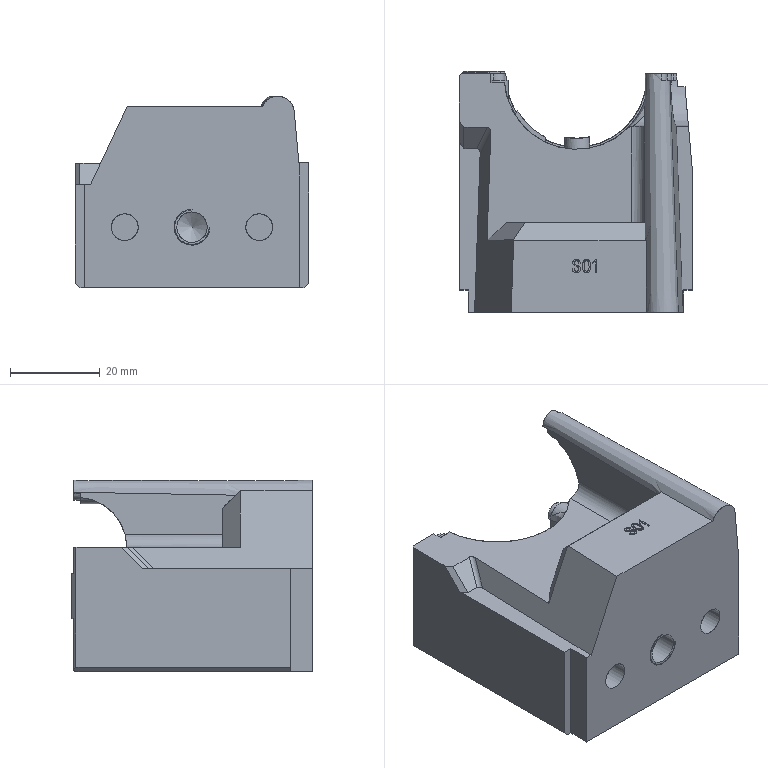NC program | PowerMill | posted with a generic post | part box 52 x 53.756 x 42.711 mm
Lines 1 to 832 of 13175:
%
O0001
N104 ( POWERMILL CB  : 2026004.0)
N105 ( POST VER      : 2026.0.0.5161)
N106 ( OPTION FILE   : FANUC)
N107 ( OUTPUT WORKPLANE : 3)
N108 (  )
N109 ( TOOL LIST )
N110 (----------------------------------)
N111 ( NO. | ID   | DIA.| TIP RAD|LENGTH)
N112 (----------------------------------)
N113 (    1|D8_4_1| 8.0 |  0.0   |108.76)
N114 (----------------------------------)
N115 (  )
N116 ( NUMBER OF TOOLPATHS: 2.0 )
N117 ( ESTIMATED PROGRAM DURATION: 0 HOURS 10 MIN 23 SEC)
N118 (  )
N119 G00 G21 G80 G40 G17
N120 G90
N121 G54
N122 G53 Z0.0
N123 (---------------)
N124 ( START TOOLPATH : 19中光-D8-偏置平坦面 )
N125 (---------------)
N126 ( TOOL NO.    :1 )
N127 ( TOOL TYPE   : ENDMILL)
N128 ( TOOL ID     : D8_4_1)
N129 ( TOOL DIA    : 8.0 LENGTH 108.76)
N130 T1
N131 M6
N132 S5000 M03
N133 G00 G90 X28.2654 Y49.6647
N134 G43 Z64.71 H1
N135
N136 G05 P10000 R8
N137 Z30.8918
N138 G01 Z27.8918 F720.0
N139 X26.6242 Y45.7769 F1200.0
N140 G03 X26.0923 Y44.9249 I0.2623 J-0.7557
N141 G01 X26.2622 Y43.8013
N142 X26.34 Y43.5763
N143 X26.6572 Y42.8315
N144 X26.7888 Y42.3169
N145 X26.86 Y41.8023
N146 X28.3026 Y0.6314
N147 Y-0.3979
N148 X28.2266 Y-0.9126
N149 X28.0887 Y-1.4272
N150 X27.8797 Y-1.9418
N151 X27.5909 Y-2.4565
N152 X27.4118 Y-2.711
N153 X27.0901 Y-3.0917
N154 X26.6667 Y-3.4857
N155 X26.3774 Y-3.7028
N156 X26.039 Y-3.9091
N157 X25.9521 Y-3.9898
N158 G00 Z49.9553
N159 G01 X-28.5374 Y-7.547 F10000.0
N160 G00 Z26.05
N161 G01 Z23.05 F720.0
N162 X-26.2828 Y-3.9798 F1200.0
N163 X-26.1415 Y-3.9873
N164 X-26.0 Y-3.9898
N165 X-24.6682
N166 X-24.8258 Y-3.9127
N167 X-25.343 Y-3.5703
N168 X-25.7171 Y-3.2493
N169 X-25.9842 Y-2.9711
N170 X-26.3774 Y-2.4524
N171 X-26.665 Y-1.9398
N172 X-26.8734 Y-1.4272
N173 X-27.012 Y-0.9126
N174 X-27.0875 Y-0.3979
N175 X-27.0858 Y0.6314
N176 X-26.0066 Y31.5474
N177 G03 X-26.5003 Y32.3145 I-0.7995 J0.0279
N178 G01 X-27.0425 Y32.5388
N179 X-27.4118 Y32.7495
N180 X-27.8904 Y33.1002
N181 X-28.3464 Y33.5439
N182 X-28.4462 Y33.6586
N183 X-29.1558 Y34.6345
N184 X-29.8427 Y35.6266
N185 X-29.9898 Y35.908
N186 G00 Z35.8914
N187 G01 X-9.4928 Y31.7865 F10000.0
N188 G00 Z30.8914
N189 G01 Z27.8914 F720.0
N190 X-9.2392 Y32.2354 Z27.8824
N191 X-9.0063 Y32.943 Z27.8694
N192 X-8.916 Y33.6824 Z27.8564
N193 X-8.9716 Y34.4253 Z27.8434
N194 X-9.1711 Y35.143 Z27.8304
N195 X-9.5067 Y35.808 Z27.8174
N196 X-9.9657 Y36.3948 Z27.8044
N197 X-10.5303 Y36.8807 Z27.7914
N198 G02 X-16.9394 Y44.3752 I10.6244 J15.5734 F1200.0
N199 G01 X-18.8601 Y48.4249
N200 X-18.9834 Y48.6399
N201 X-19.1383 Y48.8334
N202 X-19.5945 Y49.3201
N203 G03 X-22.3595 Y48.1366 I-1.1675 J-1.0941
N204 G01 X-22.2095 Y45.4574
N205 G03 X-21.5508 Y44.2512 I1.5975 J0.0895
N206 G01 X-19.7017 Y42.9115
N207 G02 X-16.0583 Y34.1909 I-5.3214 J-7.3447
N208 G01 X-16.1144 Y33.8256
N209 G03 X-14.5303 Y31.9829 I1.5815 J-0.2427
N210 G01 X-0.7665 Y32.0055
N211 G03 X-0.1268 Y32.6322 I-0.0011 J0.6409
N212 G01 X-0.1196 Y32.959
N213 G03 X-0.7159 Y33.6126 I-0.6407 J0.0142
N214 G01 X-1.2142 Y33.6473
N215 G02 X-10.5303 Y36.8807 I1.3083 J18.8068
N216 G01 X-8.4453 Y39.937
N217 G02 X-14.1271 Y47.1705 I8.5812 J12.5885
N218 G01 X-14.3504 Y47.816
N219 G02 X-14.7913 Y49.53 I15.1714 J4.8168
N220 G01 X-14.9364 Y50.2598
N221 G03 X-15.3407 Y51.0904 I-1.7837 J-0.3545
N222 G01 X-16.0194 Y51.8805
N223 G03 X-16.5057 Y52.2629 I-1.2137 J-1.0428
N224 G01 X-18.7162 Y53.3911
N225 G03 X-19.34 Y53.5627 I-0.7273 J-1.4251
N226 G01 X-24.4371 Y53.8933
N227 G03 X-26.1406 Y52.312 I-0.1036 J-1.5966
N228 G01 X-26.2339 Y42.5685
N229 G03 X-25.5124 Y41.2158 I1.5999 J-0.0154
N230 G01 X-25.0292 Y40.8984
N231 G03 X-24.2882 Y40.6417 I0.8784 J1.3374
N232 G01 X-24.0068 Y40.6174
N233 G02 X-19.791 Y35.659 I-0.3972 J-4.6091
N234 G01 X-20.3076 Y28.8359
N235 G03 X-18.7278 Y27.5514 I1.236 J-0.0935
N236 G01 X-18.19 Y27.7067
N237 X-17.161 Y24.1423
N238 X-16.7265 Y24.3046
N239 X-16.0333 Y24.4587
N240 X-14.9989 Y24.5005
N241 X7.1804 Y24.5007
N242 G03 X7.9804 Y25.3004 I0.0 J0.8
N243 G01 X7.9783 Y38.8496
N244 X7.9972 Y41.8023
N245 X8.0707 Y42.3169
N246 X8.2085 Y42.8315
N247 X8.4166 Y43.3462
N248 X8.7056 Y43.8608
N249 X9.0657 Y44.3402
N250 X9.3493 Y44.6392
N251 X9.6329 Y44.8901
N252 X9.8269 Y45.0385
N253 G03 X10.175 Y45.5347 I-0.432 J0.6733
N254 G00 Z46.126
N255 G01 X-28.6053 Y17.8571 F10000.0
N256 G00 Z30.7914
N257 G01 Z27.7914 F720.0
N258 X-24.3879 Y17.7088 F1200.0
N259 G03 X-23.8591 Y18.129 I-0.1867 J0.7779
N260 G01 X-23.6045 Y18.5751
N261 X-23.2742 Y19.0212
N262 X-23.1539 Y19.1583
N263 X-22.2398 Y19.9981
N264 X-18.5062 Y23.2754
N265 X-18.1021 Y23.6104
N266 X-17.5849 Y23.9434
N267 X-17.161 Y24.1423
N268 X-18.19 Y27.7067
N269 X-17.6522 Y27.8619
N270 G02 X-15.4248 Y28.1873 I2.3023 J-7.9753
N271 G01 X2.5454 Y28.3496
N272 G03 X4.1306 Y29.9141 I-0.0144 J1.5999
N273 G01 X4.2605 Y35.7703
N274 G03 X2.5711 Y37.4033 I-1.5996 J0.0355
N275 G01 X0.9912 Y37.3145
N276 G02 X-8.4453 Y39.937 I-0.8553 J15.211
N277 G01 X-10.5303 Y36.8807
N278 G00 Z48.65
N279 G01 X0.0231 Y5.6244 F10000.0
N280 G00 Z43.65
N281 G01 Z40.65 F720.0
N282 X-0.0299 Y6.1372 Z40.641
N283 X-0.2496 Y6.849 Z40.628
N284 X-0.6038 Y7.5043 Z40.615
N285 X-1.0792 Y8.0779 Z40.602
N286 X-1.6573 Y8.5477 Z40.589
N287 X-2.3159 Y8.8957 Z40.576
N288 X-3.0298 Y9.1086 Z40.563
N289 X-3.7715 Y9.1781 Z40.55
N290 X-6.2459 Y9.1662 F1200.0
N291 G03 X-6.9365 Y8.4611 I0.0033 J-0.694
N292 G01 X-6.9309 Y8.1127
N293 G03 X-6.2399 Y7.4298 I0.6939 J0.0111
N294 G01 X-1.298 Y7.4092
N295 G03 X-0.5991 Y8.1027 I0.0029 J0.696
N296 G01 X-0.5977 Y8.4913
N297 G03 X-1.297 Y9.1899 I-0.696 J0.0026
N298 G01 X-3.7715 Y9.1781
N299 X-3.7894 Y12.9301
N300 X-9.3072 Y12.9566
N301 G03 X-10.9133 Y11.4275 I-0.0077 J-1.5999
N302 G01 X-11.1832 Y5.3393
N303 G03 X-9.5815 Y3.6684 I1.5985 J-0.0709
N304 G01 X1.9414 Y3.6918
N305 G03 X3.5382 Y5.3034 I-0.0032 J1.6
N306 G01 X3.4946 Y11.3143
N307 G03 X1.9023 Y12.9027 I-1.6 J-0.0115
N308 G01 X-3.7894 Y12.9301
N309 X-3.8078 Y16.7917
N310 X-12.7728 Y16.8439
N311 G03 X-14.1234 Y16.1383 I-0.0095 J-1.6273
N312 G01 X-14.3703 Y15.779
N313 G03 X-14.6506 Y14.9332 I1.3186 J-0.9062
N314 G01 X-15.1584 Y1.4999
N315 G03 X-13.5589 Y-0.1605 I1.5988 J-0.0604
N316 G01 X5.8068 Y-0.1528
N317 G03 X7.4062 Y1.4563 I-0.0006 J1.6
N318 G01 X11.2566 Y1.4781
N319 X11.154 Y19.7717
N320 G03 X10.5625 Y20.5395 I-0.8 J-0.0046
N321 G01 X10.4164 Y20.5906
N322 G00 Z48.55
N323 G01 X-18.7675 Y-7.6836 F10000.0
N324 G00 Z43.55
N325 G01 Z40.55 F720.0
N326 X-16.7268 Y-3.9898 F1200.0
N327 X13.6878
N328 X13.4473 Y-3.8555
N329 X12.9301 Y-3.4925
N330 X12.6554 Y-3.25
N331 X12.3882 Y-2.9711
N332 X11.9972 Y-2.4565
N333 X11.8957 Y-2.2935
N334 X11.6697 Y-1.8603
N335 X11.4982 Y-1.4272
N336 X11.3602 Y-0.9126
N337 X11.2842 Y-0.3979
N338 X11.2566 Y1.4781
N339 X7.4062 Y1.4563
N340 X7.3285 Y15.1451
N341 G03 X5.7379 Y16.736 I-1.6 J-0.009
N342 G01 X-3.8078 Y16.7917
N343 G00 Z64.71
N344 G05 P0
N345 (---------------)
N346 ( END TOOLPATH : 19中光-D8-偏置平坦面 )
N347 (---------------)
N348 ( START TOOLPATH : 20中光-D8-等高 )
N349 (---------------)
N350 S3500 M03
N351 G00 X22.5975 Y54.6186 Z64.71
N352 G05 P10000 R8
N353 Z45.76
N354 G01 Z42.76 F2100.0
N355 G03 X22.389 Y53.8171 I1.3915 J-0.7898 F3500.0
N356 G01 X22.3949 Y53.0171
N357 X22.3978 Y52.6094
N358 X22.439 Y51.8099
N359 X22.5872 Y43.0155
N360 X23.2835 Y6.2389
N361 X23.284 Y5.8391
N362 X23.306 Y5.0396
N363 X23.3084 Y4.6399
N364 X23.3287 Y3.8404
N365 X23.3303 Y3.4406
N366 X23.3439 Y3.0409
N367 X23.3445 Y2.6411
N368 X23.359 Y2.2414
N369 X23.3907 Y0.3994
N370 X23.4044 Y-0.4005
N371 G03 X23.6325 Y-1.1967 I1.5998 J0.0276
N372 G01 X23.7083 Y-1.3228
N373 X23.7653 Y-1.3877 Z42.757
N374 X23.8412 Y-1.4283 Z42.7485
N375 X23.9806 Y-1.4727 Z42.73
N376 X24.0464 Y-1.468 Z42.7187
N377 X24.094 Y-1.4063 Z42.7047
N378 X24.0826 Y-1.3406 Z42.7
N379 G02 X23.8524 Y-0.545 I1.3695 J0.8274
N380 G01 X23.8365 Y0.2548
N381 X23.1697 Y33.8213
N382 X22.9732 Y44.2147
N383 X22.7935 Y53.0374
N384 X22.7772 Y53.8372
N385 G02 X22.9752 Y54.6414 I1.5996 J0.0326
N386 G01 X22.9943 Y54.676
N387 X23.0408 Y54.7228 Z42.6946
N388 X23.1039 Y54.7366 Z42.6803
N389 X23.1417 Y54.7335 Z42.67
N390 X23.1834 Y54.7155 Z42.6567
N391 X23.2065 Y54.6697 Z42.6442
N392 X23.1972 Y54.6235 Z42.64
N393 G03 X23.0001 Y53.8191 I1.4025 J-0.7701
N394 G01 X23.0172 Y53.0193
N395 X23.0431 Y51.8099
N396 X23.0426 Y51.4102
N397 X24.1123 Y0.1926
N398 X24.129 Y-0.6072
N399 G03 X24.36 Y-1.4026 I1.5997 J0.0334
N400 G01 X24.3927 Y-1.4565
N401 X24.4258 Y-1.4924 Z42.6364
N402 X24.4697 Y-1.5118 Z42.6264
N403 X24.5305 Y-1.5243 Z42.6098
N404 X24.5646 Y-1.5185 Z42.598
N405 X24.5863 Y-1.4844 Z42.5845
N406 X24.5785 Y-1.4489 Z42.58
N407 G02 X24.3353 Y-0.6572 I1.3558 J0.8496
N408 G01 X24.3064 Y0.1423
N409 X24.2883 Y0.6424
N410 X23.2151 Y51.8099
N411 X23.1887 Y52.2097
N412 X23.1217 Y52.6094
N413 X23.0777 Y52.7862
N414 G02 X23.0658 Y52.8824 I0.388 J0.0967
N415 G01 X23.0655 Y53.0131
N416 X23.0641 Y53.8131
N417 G02 X23.277 Y54.6135 I1.6 J0.0029
N418 G01 X23.3024 Y54.6369 Z42.5783
N419 X23.3483 Y54.6377 Z42.572
N420 X23.3792 Y54.6038 Z42.565
N421 X23.3795 Y54.5694 Z42.5622
N422 X23.0759 Y53.5774 Z42.5252
N423 X23.0541 Y53.4389 Z42.5213
N424 X23.0718 Y53.2997 Z42.52
N425 X23.1651 Y52.9591
N426 X23.261 Y52.6094
N427 X23.3278 Y52.2097
N428 X23.3541 Y51.8099
N429 X24.4789 Y0.2427
N430 X24.4766 Y0.0997
N431 X24.4642 Y-0.7002
N432 G03 X24.666 Y-1.5035 I1.5997 J-0.0249
N433 G01 X24.6866 Y-1.5404
N434 X24.7098 Y-1.5676 Z42.5162
N435 X24.7406 Y-1.5826 Z42.5056
N436 X24.779 Y-1.5917 Z42.49
N437 X24.8129 Y-1.5783 Z42.4705
N438 X24.8127 Y-1.5383 Z42.46
N439 G02 X24.6081 Y-0.7358 I1.3954 J0.7829
N440 G01 X24.618 Y0.0642
N441 X24.6201 Y0.2427
N442 X24.6055 Y0.6424
N443 X23.4815 Y51.8099
N444 X23.4731 Y51.9378
N445 X23.4204 Y52.736
N446 G02 X23.5816 Y53.5484 I1.5965 J0.1055
N447 G02 X24.3413 Y53.4198 I0.3606 J-0.1776
N448 G01 X24.6164 Y51.1796
N449 G02 X23.9136 Y50.8737 I-0.3968 J-0.0487
N450 G02 X23.5629 Y51.624 I1.2248 J1.0295
N451 G01 X23.4233 Y52.4117
N452 X23.3883 Y52.6094
N453 X23.3552 Y52.7306
N454 X23.1441 Y53.5023
N455 G02 X23.1399 Y54.3305 I1.5434 J0.422
N456 G01 X23.1812 Y54.415 Z42.4587
N457 X23.2661 Y54.4844 Z42.454
N458 X23.3797 Y54.5082 Z42.4464
N459 X23.4851 Y54.4786 Z42.4385
N460 X23.5565 Y54.4176 Z42.4323
N461 X23.7154 Y54.2153 Z42.4174
N462 X23.7968 Y54.0592 Z42.4083
N463 X23.8156 Y53.8777 Z42.4021
N464 X23.7681 Y53.708 Z42.4
N465 X23.6898 Y53.5491
N466 G03 X23.5284 Y52.7368 I1.4351 J-0.7073
N467 G01 X23.5809 Y51.9385
N468 X23.5893 Y51.8099
N469 X24.4071 Y15.8328
N470 X24.7496 Y0.2427
N471 X24.7459 Y0.0414
N472 X24.7312 Y-0.7585
N473 G03 X24.9308 Y-1.5623 I1.5997 J-0.0295
N474 G01 X24.9516 Y-1.6001
N475 X24.9877 Y-1.6386 Z42.3954
N476 X25.0367 Y-1.6542 Z42.3829
N477 X25.0812 Y-1.6562 Z42.3695
N478 X25.1281 Y-1.6296 Z42.3499
N479 X25.1259 Y-1.5731 Z42.34
N480 G02 X24.8933 Y-0.7782 I1.367 J0.8314
N481 G01 X24.875 Y0.0216
N482 X23.6911 Y51.8099
N483 X23.6809 Y51.9641
N484 X23.6284 Y52.7623
N485 G02 X23.7898 Y53.5747 I1.5966 J0.1051
N486 G01 X23.8002 Y53.5959
N487 X23.8176 Y53.6181 Z42.3354
N488 X23.8408 Y53.6294 Z42.3228
N489 X23.8603 Y53.633 Z42.31
N490 X23.8827 Y53.6221 Z42.29
N491 X23.8817 Y53.5917 Z42.28
N492 G03 X23.7196 Y52.7795 I1.4346 J-0.7085
N493 G01 X23.7715 Y51.9812
N494 X23.7826 Y51.8099
N495 X24.2532 Y31.8226
N496 X24.9795 Y0.0048
N497 X24.9978 Y-0.795
N498 G03 X25.2303 Y-1.5899 I1.5996 J0.0365
N499 G01 X25.2452 Y-1.6145
N500 X25.2647 Y-1.6357 Z42.2758
N501 X25.2892 Y-1.6463 Z42.2642
N502 X25.3139 Y-1.6503 Z42.25
N503 X25.3374 Y-1.6383 Z42.2302
N504 X25.3344 Y-1.6071 Z42.22
N505 G02 X25.1018 Y-0.8122 I1.367 J0.8316
N506 G01 X25.0834 Y-0.0124
N507 X24.638 Y19.4305
N508 X23.8648 Y51.8099
N509 X23.8528 Y51.9924
N510 X23.8003 Y52.7907
N511 G02 X23.9617 Y53.603 I1.5966 J0.105
N512 G01 X23.9704 Y53.6206
N513 X23.9873 Y53.6421 Z42.215
N514 X24.0095 Y53.6522 Z42.2015
N515 X24.0253 Y53.6543 Z42.19
N516 X24.0454 Y53.6429 Z42.1698
N517 X24.0436 Y53.614 Z42.16
N518 G03 X23.8814 Y52.8018 I1.4344 J-0.7089
N519 G01 X23.933 Y52.0035
N520 X23.9456 Y51.8099
N521 X25.18 Y0.2427
N522 X25.1814 Y-0.0288
N523 X25.1857 Y-0.8288
N524 G03 X25.4042 Y-1.6277 I1.5999 J0.0084
N525 G01 X25.4184 Y-1.6519
N526 X25.4408 Y-1.676 Z42.1555
N527 X25.4698 Y-1.6866 Z42.1431
N528 X25.4954 Y-1.6888 Z42.1298
N529 X25.5223 Y-1.6734 Z42.11
N530 X25.5192 Y-1.6382 Z42.1
N531 G02 X25.2858 Y-0.8435 I1.3661 J0.8329
N532 G01 X25.2667 Y-0.0437
N533 X24.305 Y40.2173
N534 X24.0175 Y51.8099
N535 X24.0041 Y52.0135
N536 X23.9516 Y52.8118
N537 G02 X24.1129 Y53.6241 I1.5965 J0.105
N538 G01 X24.1198 Y53.638
N539 X24.1351 Y53.6578 Z42.0947
N540 X24.1544 Y53.6667 Z42.0804
N541 X24.1658 Y53.668 Z42.07
N542 X24.1818 Y53.6575 Z42.0497
N543 X24.1791 Y53.6314 Z42.04
N544 G03 X24.0177 Y52.8191 I1.4352 J-0.7073
N545 G01 X24.0702 Y52.0208
N546 X24.0841 Y51.8099
N547 X24.937 Y17.4318
N548 X25.3523 Y-0.053
N549 X25.3713 Y-0.8528
N550 G03 X25.6046 Y-1.6475 I1.5995 J0.038
N551 G01 X25.615 Y-1.6645
N552 X25.6333 Y-1.6841 Z42.0351
N553 X25.6556 Y-1.6923 Z42.0218
N554 X25.6716 Y-1.6934 Z42.01
N555 X25.6903 Y-1.6809 Z41.9899
N556 X25.686 Y-1.6528 Z41.98
N557 G02 X25.453 Y-0.858 I1.3666 J0.8322
N558 G01 X25.4343 Y-0.0583
N559 X25.2683 Y7.0384
N560 X24.1507 Y51.8099
N561 X24.1363 Y52.0262
N562 X24.0832 Y52.8245
N563 G02 X24.244 Y53.6369 I1.5965 J0.1062
N564 G01 X24.2515 Y53.6522
N565 X24.2696 Y53.6744 Z41.9746
N566 X24.2934 Y53.6835 Z41.9602
N567 X24.3074 Y53.6842 Z41.9499
N568 X24.3276 Y53.6709 Z41.9296
N569 X24.3253 Y53.6409 Z41.92
N570 G03 X24.1547 Y52.8305 I1.4271 J-0.7236
N571 G01 X24.1981 Y52.0316
N572 X24.2102 Y51.8099
N573 X24.4577 Y42.216
N574 X25.5066 Y0.2427
N575 X25.508 Y-0.0632
N576 X25.5119 Y-0.8632
N577 G03 X25.7301 Y-1.6622 I1.5999 J0.0077
N578 G01 X25.7411 Y-1.6811
N579 X25.7635 Y-1.7045 Z41.9149
N580 X25.7921 Y-1.7131 Z41.9012
N581 X25.8118 Y-1.713 Z41.8898
N582 X25.8361 Y-1.6962 Z41.8698
N583 X25.8321 Y-1.6622 Z41.86
N584 G02 X25.5979 Y-0.8678 I1.3652 J0.8343
N585 G01 X25.5779 Y-0.068
N586 X24.7435 Y33.4216
N587 X24.2647 Y51.8099
N588 X24.2499 Y52.0357
N589 X24.1976 Y52.834
N590 G02 X24.3592 Y53.6463 I1.5966 J0.1046
N591 G01 X24.3646 Y53.6574
N592 X24.3789 Y53.6762 Z41.8543
N593 X24.3962 Y53.6843 Z41.8391
N594 X24.4045 Y53.685 Z41.83
N595 X24.4174 Y53.6749 Z41.8095
N596 X24.4138 Y53.6508 Z41.8
N597 G03 X24.252 Y52.8385 I1.4348 J-0.7081
N598 G01 X24.3041 Y52.0402
N599 X24.3191 Y51.8099
N600 X25.1215 Y21.0295
N601 X25.6492 Y-0.0692
N602 X25.6693 Y-0.8689
N603 G03 X25.9035 Y-1.6633 I1.5995 J0.04
N604 G01 X25.9078 Y-1.6704
N605 X25.9211 Y-1.6865 Z41.7936
N606 X25.9338 Y-1.6932 Z41.7771
N607 X25.9376 Y-1.6934 Z41.7701
N608 X25.9434 Y-1.6847 Z41.7494
N609 X25.9366 Y-1.6646 Z41.74
N610 G02 X25.7177 Y-0.8659 I1.381 J0.8079
N611 G01 X25.7131 Y-0.0659
N612 X25.7113 Y0.2427
N613 X25.5103 Y8.2376
N614 X24.3717 Y51.8099
N615 X24.3561 Y52.0447
N616 X24.3031 Y52.8429
N617 G02 X24.4639 Y53.6554 I1.5964 J0.1061
N618 G01 X24.4688 Y53.6652
N619 X24.4819 Y53.6832 Z41.7341
N620 X24.4971 Y53.6912 Z41.7186
N621 X24.5038 Y53.6919 Z41.71
N622 X24.5142 Y53.6828 Z41.6895
N623 X24.5101 Y53.6604 Z41.68
N624 G03 X24.3488 Y52.848 I1.4352 J-0.7072
N625 G01 X24.4014 Y52.0497
N626 X24.4172 Y51.8099
N627 X24.7096 Y41.0168
N628 X25.774 Y0.2427
N629 X25.7757 Y-0.0626
N630 X25.7801 Y-0.8626
N631 G03 X25.9988 Y-1.6614 I1.6 J0.0088
N632 G01 X26.0072 Y-1.6757
N633 X26.0295 Y-1.6984 Z41.6743
N634 X26.0573 Y-1.7051 Z41.6594
N635 X26.0718 Y-1.7037 Z41.6498
N636 X26.0933 Y-1.6861 Z41.6295
N637 X26.0885 Y-1.6533 Z41.62
N638 G02 X25.8535 Y-0.8592 I1.3644 J0.8357
N639 G01 X25.8327 Y-0.0594
N640 X25.0048 Y31.8226
N641 X24.4616 Y51.8099
N642 X24.4455 Y52.0547
N643 X24.3929 Y52.8529
N644 G02 X24.5542 Y53.6653 I1.5966 J0.1052
N645 G01 X24.5589 Y53.6748
N646 X24.5718 Y53.6926 Z41.6141
N647 X24.5865 Y53.7005 Z41.5985
N648 X24.5927 Y53.7012 Z41.59
N649 X24.6026 Y53.6923 Z41.5695
N650 X24.5983 Y53.6702 Z41.56
N651 G03 X24.437 Y52.8579 I1.4352 J-0.7072
N652 G01 X24.4896 Y52.0596
N653 X24.5061 Y51.8099
N654 X25.3218 Y21.829
N655 X25.889 Y0.2427
N656 X25.8916 Y-0.0563
N657 X25.8985 Y-0.8562
N658 G03 X26.1197 Y-1.6543 I1.5999 J0.0138
N659 G01 X26.1251 Y-1.6634
N660 X26.1409 Y-1.6811 Z41.5539
N661 X26.1585 Y-1.6873 Z41.538
N662 X26.1652 Y-1.687 Z41.53
N663 X26.1764 Y-1.6754 Z41.5094
N664 X26.1707 Y-1.6517 Z41.5
N665 G02 X25.9499 Y-0.8534 I1.3791 J0.8113
N666 G01 X25.9434 Y-0.0534
N667 X25.9409 Y0.2427
N668 X25.6056 Y13.0345
N669 X24.547 Y51.8099
N670 X24.5303 Y52.0642
N671 X24.4776 Y52.8625
N672 G02 X24.6389 Y53.6749 I1.5966 J0.1052
N673 G01 X24.6429 Y53.6828
N674 X24.655 Y53.7003 Z41.4938
N675 X24.6681 Y53.708 Z41.4776
N676 X24.6727 Y53.7085 Z41.47
N677 X24.6804 Y53.7001 Z41.4494
N678 X24.6754 Y53.6791 Z41.44
N679 G03 X24.5139 Y52.8668 I1.4351 J-0.7075
N680 G01 X24.5663 Y52.0685
N681 X24.5833 Y51.8099
N682 X24.8889 Y41.0168
N683 X25.9965 Y0.2427
N684 X25.998 Y-0.0512
N685 X26.0022 Y-0.8512
N686 G03 X26.2208 Y-1.6501 I1.6001 J0.0084
N687 G01 X26.2261 Y-1.6591
N688 X26.2418 Y-1.6769 Z41.4339
N689 X26.2594 Y-1.6831 Z41.418
N690 X26.2662 Y-1.6828 Z41.41
N691 X26.2774 Y-1.6713 Z41.3894
N692 X26.2718 Y-1.6476 Z41.38
N693 G02 X26.0519 Y-0.8491 I1.3801 J0.8096
N694 G01 X26.0463 Y-0.0491
N695 X26.0443 Y0.2427
N696 X25.1184 Y34.2211
N697 X24.619 Y51.8099
N698 X24.6049 Y52.0729
N699 X24.562 Y52.8718
N700 G02 X24.7332 Y53.6821 I1.5978 J0.0857
N701 G01 X24.7354 Y53.6865
N702 X24.7453 Y53.7037 Z41.3729
N703 X24.7523 Y53.7119 Z41.3548
N704 X24.7533 Y53.7124 Z41.35
N705 X24.7534 Y53.7059 Z41.3291
N706 X24.7458 Y53.6876 Z41.32
N707 G03 X24.5845 Y52.8752 I1.4352 J-0.7071
N708 G01 X24.6371 Y52.077
N709 X24.6548 Y51.8099
N710 X25.3814 Y26.2262
N711 X26.0951 Y-0.047
N712 X26.1169 Y-0.8467
N713 G03 X26.3529 Y-1.6406 I1.5994 J0.0435
N714 G01 X26.3578 Y-1.6486
N715 X26.3727 Y-1.6654 Z41.3138
N716 X26.3885 Y-1.6714 Z41.2976
N717 X26.394 Y-1.6711 Z41.29
N718 X26.4028 Y-1.6606 Z41.2694
N719 X26.3963 Y-1.6386 Z41.26
N720 G02 X26.1603 Y-0.8447 I1.3634 J0.8372
N721 G01 X26.1387 Y-0.045
N722 X25.622 Y19.0307
N723 X24.6877 Y51.8099
N724 X24.6701 Y52.0796
N725 X24.6181 Y52.8779
N726 G02 X24.7799 Y53.6902 I1.5966 J0.1041
N727 G01 X24.7949 Y53.7095 Z41.2512
N728 X24.8096 Y53.7128 Z41.23
N729 X24.8099 Y53.7127 Z41.2293
N730 X24.8157 Y53.6983 Z41.2085
N731 X24.8093 Y53.6748 Z41.2
N732 X24.8089 Y53.674
N733 G03 X24.6473 Y52.8617 I1.435 J-0.7077
N734 G01 X24.6995 Y52.0634
N735 X24.7161 Y51.8099
N736 X25.1246 Y37.8188
N737 X25.8739 Y11.4356
N738 X26.18 Y0.2427
N739 X26.1819 Y-0.043
N740 X26.1873 Y-0.843
N741 G03 X26.407 Y-1.6415 I1.6 J0.0107
N742 G01 X26.4116 Y-1.6493
N743 X26.4262 Y-1.6665 Z41.1937
N744 X26.4418 Y-1.6727 Z41.1773
N745 X26.4471 Y-1.6725 Z41.17
N746 X26.456 Y-1.662 Z41.1494
N747 X26.4499 Y-1.6398 Z41.14
N748 G02 X26.2312 Y-0.841 I1.3812 J0.8076
N749 G01 X26.2268 Y-0.041
N750 X26.2253 Y0.2427
N751 X25.1589 Y37.8188
N752 X24.7442 Y51.8099
N753 X24.7286 Y52.0473
N754 X24.676 Y52.8456
N755 G02 X24.8374 Y53.6579 I1.5966 J0.105
N756 G01 X24.8523 Y53.6772 Z41.1312
N757 X24.8668 Y53.6805 Z41.11
N758 X24.8671 Y53.6803 Z41.1092
N759 X24.8727 Y53.6661 Z41.0885
N760 X24.8663 Y53.6426 Z41.08
N761 X24.8659 Y53.6418
N762 G03 X24.7048 Y52.8294 I1.4354 J-0.7068
N763 G01 X24.7576 Y52.0311
N764 X24.7722 Y51.8099
N765 X25.389 Y31.0231
N766 X26.2645 Y0.2427
N767 X26.267 Y-0.0382
N768 X26.274 Y-0.8382
N769 G03 X26.4954 Y-1.6363 I1.6 J0.0141
N770 G01 X26.5016 Y-1.6467
N771 X26.521 Y-1.6668 Z41.0739
N772 X26.544 Y-1.6725 Z41.0581
N773 X26.5536 Y-1.6712 Z41.0498
N774 X26.5697 Y-1.6559 Z41.0294
N775 X26.5641 Y-1.6278 Z41.02
N776 G02 X26.3272 Y-0.8342 I1.3625 J0.8388
N777 G01 X26.3046 Y-0.0345
N778 X25.607 Y24.6272
N779 X24.7991 Y51.8099
N780 X24.7856 Y52.015
N781 X24.7329 Y52.8133
N782 G02 X24.8941 Y53.6257 I1.5965 J0.1054
N783 G01 X24.9079 Y53.6443 Z41.0111
N784 X24.9207 Y53.6475 Z40.99
N785 X24.9213 Y53.6471 Z40.9883
N786 X24.9253 Y53.6335 Z40.9682
N787 X24.9187 Y53.6113 Z40.96
N788 X24.9179 Y53.6097
N789 G03 X24.7562 Y52.7974 I1.435 J-0.7078
N790 G01 X24.8085 Y51.9991
N791 X24.8209 Y51.8099
N792 X25.0298 Y45.0142
N793 X25.9511 Y13.834
N794 X26.3401 Y-0.0309
N795 X26.3625 Y-0.8306
N796 G03 X26.5992 Y-1.6243 I1.5994 J0.0449
N797 G01 X26.6001 Y-1.6256
N798 X26.6112 Y-1.6431 Z40.9518
N799 X26.6168 Y-1.6506 Z40.9316
N800 X26.6169 Z40.93
N801 X26.6137 Y-1.6435 Z40.9089
N802 X26.6036 Y-1.6254 Z40.9
N803 G02 X26.3825 Y-0.8273 I1.3788 J0.8116
N804 G01 X26.3758 Y-0.0273
N805 X26.3735 Y0.2427
N806 X26.043 Y11.8353
N807 X25.2006 Y40.2173
N808 X24.8419 Y51.8099
N809 X24.8304 Y51.9832
N810 X24.7773 Y52.7814
N811 G02 X24.938 Y53.5939 I1.5964 J0.1062
N812 G01 X24.9516 Y53.6123 Z40.8911
N813 X24.9637 Y53.6155 Z40.87
N814 X24.9645 Y53.615 Z40.868
N815 X24.9679 Y53.6017 Z40.8481
N816 X24.9613 Y53.5799 Z40.84
N817 X24.9603 Y53.578
N818 G03 X24.7994 Y52.7655 I1.4356 J-0.7065
N819 G01 X24.8524 Y51.9673
N820 X24.8629 Y51.8099
N821 X25.5025 Y31.0231
N822 X26.4098 Y0.2427
N823 X26.4115 Y-0.0237
N824 X26.4166 Y-0.8237
N825 G03 X26.636 Y-1.6223 I1.5999 J0.0101
N826 G01 X26.6395 Y-1.6283
N827 X26.654 Y-1.6455 Z40.8332
N828 X26.6688 Y-1.6512 Z40.8159
N829 X26.6725 Y-1.6508 Z40.81
N830 X26.6798 Y-1.64 Z40.7892
N831 X26.6731 Y-1.6183 Z40.78
N832 G02 X26.4523 Y-0.82 I1.3792 J0.8111
N833 G01 X26.4459 Y-0.0201
N834 X26.4438 Y0.2427
N835 X25.5781 Y29.4241
N836 X24.8741 Y51.9514
N837 X24.8492 Y52.751
N838 G02 X25.0384 Y53.5573 I1.5992 J0.05
N839 G01 X25.0513 Y53.5747 Z40.771
N840 X25.0613 Y53.5776 Z40.75
N841 X25.062 Y53.5769 Z40.7471
N842 X25.0631 Y53.5645 Z40.7278
N843 X25.0554 Y53.5443 Z40.72
N844 X25.054 Y53.5416
N845 G03 X24.8661 Y52.735 I1.4112 J-0.7539
N846 G01 X24.8925 Y51.9354
N847 X25.0416 Y47.4127
N848 X25.7606 Y24.2274
N849 X26.4728 Y0.2427
N850 X26.475 Y-0.0167
N851 X26.4816 Y-0.8166
N852 G03 X26.7025 Y-1.6148 I1.5999 J0.0132
N853 G01 X26.7054 Y-1.6198
N854 X26.7193 Y-1.6367 Z40.713
N855 X26.7325 Y-1.6424 Z40.6951
N856 X26.7351 Y-1.6421 Z40.69
N857 X26.7406 Y-1.6319 Z40.6692
N858 X26.7334 Y-1.6111 Z40.66
N859 G02 X26.5114 Y-0.8132 I1.3779 J0.8132
N860 G01 X26.5037 Y-0.0132
N861 X26.5013 Y0.2427
N862 X25.931 Y19.4305
N863 X25.1742 Y43.815
N864 X24.9079 Y51.9197
N865 X24.8816 Y52.7193
N866 G02 X25.0696 Y53.5259 I1.5992 J0.0525
N867 G01 X25.0825 Y53.5433 Z40.651
N868 X25.0925 Y53.5462 Z40.63
N869 X25.0933 Y53.5455 Z40.6271
N870 X25.0944 Y53.5331 Z40.6078
N871 X25.0867 Y53.5129 Z40.6
N872 X25.0852 Y53.5102
N873 G03 X24.8972 Y52.7036 I1.4111 J-0.7543
N874 G01 X24.9234 Y51.904
N875 X25.3191 Y39.8175
N876 X26.1257 Y13.834
N877 X26.5325 Y-0.0098
N878 X26.556 Y-0.8095
N879 G03 X26.7938 Y-1.6029 I1.5993 J0.047
N880 G01 X26.7968 Y-1.6077
N881 X26.8106 Y-1.6241 Z40.593
N882 X26.8232 Y-1.6298 Z40.5751
N883 X26.8257 Y-1.6295 Z40.57
N884 X26.8303 Y-1.6197 Z40.5492
N885 X26.8225 Y-1.5995 Z40.54
N886 G02 X26.5849 Y-0.8061 I1.3617 J0.8402
N887 G01 X26.5615 Y-0.0064
N888 X26.3086 Y8.6373
N889 X25.5021 Y34.6208
N890 X24.9389 Y51.8883
N891 X24.9128 Y52.6879
N892 G02 X25.101 Y53.4944 I1.5991 J0.0521
N893 G01 X25.1137 Y53.5118 Z40.531
N894 X25.1234 Y53.5147 Z40.51
N895 X25.1241 Y53.5139 Z40.5069
N896 X25.125 Y53.5016 Z40.4877
N897 X25.1173 Y53.4816 Z40.48
N898 X25.1158 Y53.4787
N899 G03 X24.9276 Y52.6722 I1.4109 J-0.7544
N900 G01 X24.9537 Y51.8726
N901 X25.647 Y30.6234
N902 X26.5871 Y0.2427
N903 X26.5889 Y-0.005
N904 X26.5947 Y-0.805
N905 G03 X26.8149 Y-1.6034 I1.6 J0.0117
N906 G01 X26.8175 Y-1.6078
N907 X26.8301 Y-1.6244 Z40.4728
N908 X26.841 Y-1.6308 Z40.4547
N909 X26.8429 Y-1.6307 Z40.45
N910 X26.846 Y-1.6219 Z40.4291
N911 X26.8382 Y-1.6024 Z40.42
N912 G02 X26.6186 Y-0.8039 I1.3804 J0.8091
N913 G01 X26.6133 Y-0.0039
N914 X26.6116 Y0.2427
N915 X25.8301 Y25.4267
N916 X25.1288 Y47.013
N917 X24.9632 Y51.8568
N918 X24.9359 Y52.6563
N919 G02 X25.1228 Y53.4632 I1.5991 J0.0547
N920 G01 X25.1345 Y53.4801 Z40.4109
N921 X25.1423 Y53.4829 Z40.39
N922 X25.143 Y53.4818 Z40.3858
N923 X25.1423 Y53.4702 Z40.3673
N924 X25.1344 Y53.4512 Z40.36
N925 X25.1323 Y53.4473
N926 G03 X24.9453 Y52.6405 I1.412 J-0.7523
N927 G01 X24.9725 Y51.841
N928 X25.2866 Y42.6158
N929 X25.9878 Y21.0295